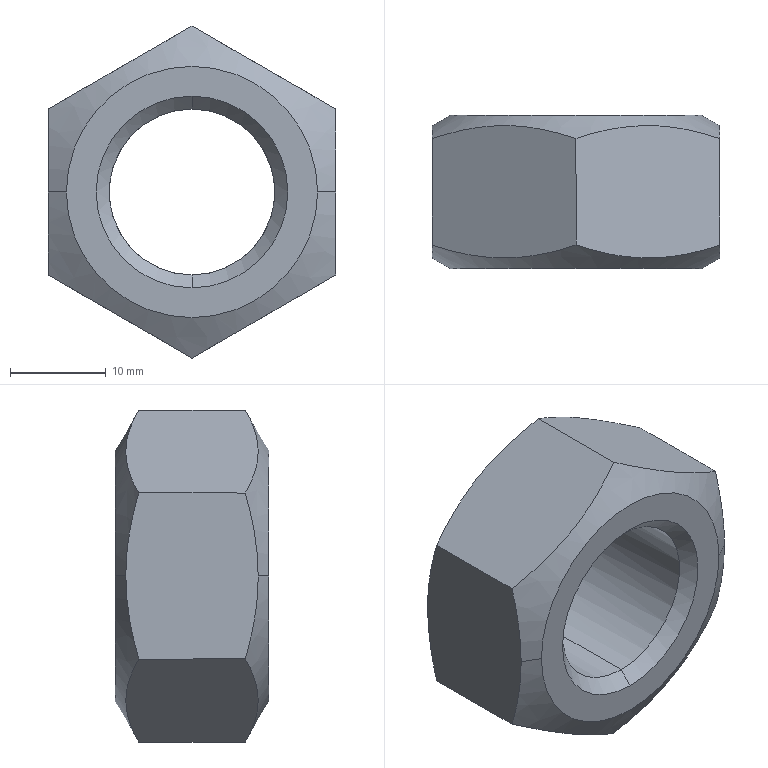Part | SolidWorks | features BaseBody 1 | 1 solid | 18 faces | box 30 x 16 x 34.641 mm | volume 8202 mm3 | cone 8 | plane 8 | cylinder 2 | commonest cylinder face diameters 17.294 x2
STEP:
#1=CARTESIAN_POINT('',(0.,94.353,-8.647));
#2=VERTEX_POINT('',#1);
#3=CARTESIAN_POINT('',(0.,94.353,8.647));
#4=VERTEX_POINT('',#3);
#5=CARTESIAN_POINT('',(0.,94.353,0.));
#6=DIRECTION('',(0.,1.,0.));
#7=DIRECTION('',(0.,0.,1.));
#8=AXIS2_PLACEMENT_3D('',#5,#6,#7);
#9=CIRCLE('',#8,8.647);
#10=EDGE_CURVE('',#2,#4,#9,.T.);
#11=ORIENTED_EDGE('',*,*,#10,.F.);
#12=CARTESIAN_POINT('',(0.,107.647,-8.647));
#13=VERTEX_POINT('',#12);
#14=CARTESIAN_POINT('',(0.,500.,-8.647));
#15=DIRECTION('',(0.,1.,0.));
#16=VECTOR('',#15,1000.);
#17=LINE('',#14,#16);
#18=EDGE_CURVE('',#2,#13,#17,.T.);
#19=ORIENTED_EDGE('',*,*,#18,.T.);
#20=CARTESIAN_POINT('',(-8.647,107.647,0.));
#21=VERTEX_POINT('',#20);
#22=CARTESIAN_POINT('',(0.,107.647,0.));
#23=DIRECTION('',(0.,-1.,0.));
#24=DIRECTION('',(0.,0.,1.));
#25=AXIS2_PLACEMENT_3D('',#22,#23,#24);
#26=CIRCLE('',#25,8.647);
#27=EDGE_CURVE('',#21,#13,#26,.T.);
#28=ORIENTED_EDGE('',*,*,#27,.F.);
#29=CARTESIAN_POINT('',(0.,107.647,8.647));
#30=VERTEX_POINT('',#29);
#31=CARTESIAN_POINT('',(0.,107.647,0.));
#32=DIRECTION('',(0.,-1.,0.));
#33=DIRECTION('',(0.,0.,1.));
#34=AXIS2_PLACEMENT_3D('',#31,#32,#33);
#35=CIRCLE('',#34,8.647);
#36=EDGE_CURVE('',#30,#21,#35,.T.);
#37=ORIENTED_EDGE('',*,*,#36,.F.);
#38=CARTESIAN_POINT('',(0.,500.,8.647));
#39=DIRECTION('',(0.,1.,0.));
#40=VECTOR('',#39,1000.);
#41=LINE('',#38,#40);
#42=EDGE_CURVE('',#4,#30,#41,.T.);
#43=ORIENTED_EDGE('',*,*,#42,.F.);
#44=EDGE_LOOP('',(#11,#19,#28,#37,#43));
#45=FACE_OUTER_BOUND('',#44,.T.);
#46=CARTESIAN_POINT('',(0.,500.,0.));
#47=DIRECTION('',(0.,1.,0.));
#48=DIRECTION('',(0.,0.,1.));
#49=AXIS2_PLACEMENT_3D('',#46,#47,#48);
#50=CYLINDRICAL_SURFACE('',#49,8.647);
#51=ADVANCED_FACE('',(#45),#50,.F.);
#52=ORIENTED_EDGE('',*,*,#10,.T.);
#53=CARTESIAN_POINT('',(0.,93.,10.));
#54=VERTEX_POINT('',#53);
#55=CARTESIAN_POINT('',(0.,93.,10.));
#56=DIRECTION('',(0.,-0.7071,0.7071));
#57=VECTOR('',#56,1000.);
#58=LINE('',#55,#57);
#59=EDGE_CURVE('',#4,#54,#58,.T.);
#60=ORIENTED_EDGE('',*,*,#59,.T.);
#61=CARTESIAN_POINT('',(0.,93.,-10.));
#62=VERTEX_POINT('',#61);
#63=CARTESIAN_POINT('',(0.,93.,0.));
#64=DIRECTION('',(0.,1.,0.));
#65=DIRECTION('',(0.,0.,-1.));
#66=AXIS2_PLACEMENT_3D('',#63,#64,#65);
#67=CIRCLE('',#66,10.);
#68=EDGE_CURVE('',#62,#54,#67,.T.);
#69=ORIENTED_EDGE('',*,*,#68,.F.);
#70=CARTESIAN_POINT('',(0.,93.,-10.));
#71=DIRECTION('',(0.,-0.7071,-0.7071));
#72=VECTOR('',#71,1000.);
#73=LINE('',#70,#72);
#74=EDGE_CURVE('',#2,#62,#73,.T.);
#75=ORIENTED_EDGE('',*,*,#74,.F.);
#76=EDGE_LOOP('',(#52,#60,#69,#75));
#77=FACE_OUTER_BOUND('',#76,.T.);
#78=CARTESIAN_POINT('',(0.,93.,0.));
#79=DIRECTION('',(0.,-1.,0.));
#80=DIRECTION('',(0.,0.,-1.));
#81=AXIS2_PLACEMENT_3D('',#78,#79,#80);
#82=CONICAL_SURFACE('',#81,10.,0.7854);
#83=ADVANCED_FACE('',(#77),#82,.F.);
#84=ORIENTED_EDGE('',*,*,#27,.T.);
#85=CARTESIAN_POINT('',(8.647,107.647,0.));
#86=VERTEX_POINT('',#85);
#87=CARTESIAN_POINT('',(0.,107.647,0.));
#88=DIRECTION('',(0.,-1.,0.));
#89=DIRECTION('',(0.,0.,1.));
#90=AXIS2_PLACEMENT_3D('',#87,#88,#89);
#91=CIRCLE('',#90,8.647);
#92=EDGE_CURVE('',#13,#86,#91,.T.);
#93=ORIENTED_EDGE('',*,*,#92,.T.);
#94=CARTESIAN_POINT('',(10.,109.,0.));
#95=VERTEX_POINT('',#94);
#96=CARTESIAN_POINT('',(10.,109.,0.));
#97=DIRECTION('',(0.7071,0.7071,0.));
#98=VECTOR('',#97,1000.);
#99=LINE('',#96,#98);
#100=EDGE_CURVE('',#86,#95,#99,.T.);
#101=ORIENTED_EDGE('',*,*,#100,.T.);
#102=CARTESIAN_POINT('',(-10.,109.,0.));
#103=VERTEX_POINT('',#102);
#104=CARTESIAN_POINT('',(0.,109.,0.));
#105=DIRECTION('',(0.,-1.,0.));
#106=DIRECTION('',(-1.,0.,0.));
#107=AXIS2_PLACEMENT_3D('',#104,#105,#106);
#108=CIRCLE('',#107,10.);
#109=EDGE_CURVE('',#103,#95,#108,.T.);
#110=ORIENTED_EDGE('',*,*,#109,.F.);
#111=CARTESIAN_POINT('',(-10.,109.,0.));
#112=DIRECTION('',(-0.7071,0.7071,0.));
#113=VECTOR('',#112,1000.);
#114=LINE('',#111,#113);
#115=EDGE_CURVE('',#21,#103,#114,.T.);
#116=ORIENTED_EDGE('',*,*,#115,.F.);
#117=EDGE_LOOP('',(#84,#93,#101,#110,#116));
#118=FACE_OUTER_BOUND('',#117,.T.);
#119=CARTESIAN_POINT('',(0.,109.,0.));
#120=DIRECTION('',(0.,1.,0.));
#121=DIRECTION('',(-1.,0.,0.));
#122=AXIS2_PLACEMENT_3D('',#119,#120,#121);
#123=CONICAL_SURFACE('',#122,10.,0.7854);
#124=ADVANCED_FACE('',(#118),#123,.F.);
#125=CARTESIAN_POINT('',(13.1,93.,0.));
#126=VERTEX_POINT('',#125);
#127=CARTESIAN_POINT('',(-13.1,93.,0.));
#128=VERTEX_POINT('',#127);
#129=CARTESIAN_POINT('',(0.,93.,0.));
#130=DIRECTION('',(0.,-1.,0.));
#131=DIRECTION('',(-1.,0.,0.));
#132=AXIS2_PLACEMENT_3D('',#129,#130,#131);
#133=CIRCLE('',#132,13.1);
#134=EDGE_CURVE('',#126,#128,#133,.T.);
#135=ORIENTED_EDGE('',*,*,#134,.F.);
#136=CARTESIAN_POINT('',(15.,94.097,0.));
#137=VERTEX_POINT('',#136);
#138=CARTESIAN_POINT('',(17.346,95.451,0.));
#139=DIRECTION('',(0.866,0.5,0.));
#140=VECTOR('',#139,1000.);
#141=LINE('',#138,#140);
#142=EDGE_CURVE('',#126,#137,#141,.T.);
#143=ORIENTED_EDGE('',*,*,#142,.T.);
#144=CARTESIAN_POINT('',(15.,95.437,8.66));
#145=VERTEX_POINT('',#144);
#146=CARTESIAN_POINT('',(15.,94.097,0.));
#147=CARTESIAN_POINT('',(15.,94.097,0.735));
#148=CARTESIAN_POINT('',(15.,94.129,1.473));
#149=CARTESIAN_POINT('',(15.,94.251,2.934));
#150=CARTESIAN_POINT('',(15.,94.342,3.659));
#151=CARTESIAN_POINT('',(15.,94.692,5.822));
#152=CARTESIAN_POINT('',(15.,95.029,7.247));
#153=CARTESIAN_POINT('',(15.,95.437,8.66));
#154=B_SPLINE_CURVE_WITH_KNOTS('',3,(#146,#147,#148,#149,#150,#151,#152,#153),.UNSPECIFIED.,.F.,.F.,(4,2,2,4),(0.008763,0.01095,0.01313,0.01749),.UNSPECIFIED.);
#155=EDGE_CURVE('',#137,#145,#154,.T.);
#156=ORIENTED_EDGE('',*,*,#155,.T.);
#157=CARTESIAN_POINT('',(0.000000043,95.437,17.321));
#158=VERTEX_POINT('',#157);
#159=CARTESIAN_POINT('',(15.,95.437,8.66));
#160=CARTESIAN_POINT('',(13.775,95.029,9.367));
#161=CARTESIAN_POINT('',(12.542,94.692,10.079));
#162=CARTESIAN_POINT('',(10.049,94.226,11.519));
#163=CARTESIAN_POINT('',(8.79,94.098,12.246));
#164=CARTESIAN_POINT('',(6.877,94.097,13.35));
#165=CARTESIAN_POINT('',(6.236,94.128,13.72));
#166=CARTESIAN_POINT('',(4.969,94.25,14.452));
#167=CARTESIAN_POINT('',(4.339,94.341,14.815));
#168=CARTESIAN_POINT('',(2.463,94.691,15.899));
#169=CARTESIAN_POINT('',(1.226,95.028,16.613));
#170=CARTESIAN_POINT('',(0.000000043,95.437,17.321));
#171=B_SPLINE_CURVE_WITH_KNOTS('',3,(#159,#160,#161,#162,#163,#164,#165,#166,#167,#168,#169,#170),.UNSPECIFIED.,.F.,.F.,(4,2,2,2,2,4),(0.,0.004373,0.008746,0.01093,0.01312,0.01749),.UNSPECIFIED.);
#172=EDGE_CURVE('',#145,#158,#171,.T.);
#173=ORIENTED_EDGE('',*,*,#172,.T.);
#174=CARTESIAN_POINT('',(-15.,95.437,8.66));
#175=VERTEX_POINT('',#174);
#176=CARTESIAN_POINT('',(0.000000043,95.437,17.321));
#177=CARTESIAN_POINT('',(-1.225,95.029,16.613));
#178=CARTESIAN_POINT('',(-2.458,94.692,15.901));
#179=CARTESIAN_POINT('',(-4.951,94.226,14.462));
#180=CARTESIAN_POINT('',(-6.21,94.098,13.735));
#181=CARTESIAN_POINT('',(-8.123,94.097,12.631));
#182=CARTESIAN_POINT('',(-8.764,94.128,12.261));
#183=CARTESIAN_POINT('',(-10.031,94.25,11.529));
#184=CARTESIAN_POINT('',(-10.661,94.341,11.166));
#185=CARTESIAN_POINT('',(-12.537,94.691,10.082));
#186=CARTESIAN_POINT('',(-13.774,95.028,9.368));
#187=CARTESIAN_POINT('',(-15.,95.437,8.66));
#188=B_SPLINE_CURVE_WITH_KNOTS('',3,(#176,#177,#178,#179,#180,#181,#182,#183,#184,#185,#186,#187),.UNSPECIFIED.,.F.,.F.,(4,2,2,2,2,4),(0.,0.004373,0.008746,0.01093,0.01312,0.01749),.UNSPECIFIED.);
#189=EDGE_CURVE('',#158,#175,#188,.T.);
#190=ORIENTED_EDGE('',*,*,#189,.T.);
#191=CARTESIAN_POINT('',(-15.,94.097,0.));
#192=VERTEX_POINT('',#191);
#193=CARTESIAN_POINT('',(-15.,95.437,8.66));
#194=CARTESIAN_POINT('',(-15.,95.028,7.244));
#195=CARTESIAN_POINT('',(-15.,94.691,5.816));
#196=CARTESIAN_POINT('',(-15.,94.225,2.933));
#197=CARTESIAN_POINT('',(-15.,94.097,1.475));
#198=CARTESIAN_POINT('',(-15.,94.097,0.));
#199=B_SPLINE_CURVE_WITH_KNOTS('',3,(#193,#194,#195,#196,#197,#198),.UNSPECIFIED.,.F.,.F.,(4,2,4),(0.,0.004381,0.008763),.UNSPECIFIED.);
#200=EDGE_CURVE('',#175,#192,#199,.T.);
#201=ORIENTED_EDGE('',*,*,#200,.T.);
#202=CARTESIAN_POINT('',(-17.346,95.451,0.));
#203=DIRECTION('',(-0.866,0.5,0.));
#204=VECTOR('',#203,1000.);
#205=LINE('',#202,#204);
#206=EDGE_CURVE('',#128,#192,#205,.T.);
#207=ORIENTED_EDGE('',*,*,#206,.F.);
#208=EDGE_LOOP('',(#135,#143,#156,#173,#190,#201,#207));
#209=FACE_OUTER_BOUND('',#208,.T.);
#210=CARTESIAN_POINT('',(0.,95.451,0.));
#211=DIRECTION('',(0.,1.,0.));
#212=DIRECTION('',(-1.,0.,0.));
#213=AXIS2_PLACEMENT_3D('',#210,#211,#212);
#214=CONICAL_SURFACE('',#213,17.346,1.047);
#215=ADVANCED_FACE('',(#209),#214,.T.);
#216=CARTESIAN_POINT('',(-13.1,109.,0.));
#217=VERTEX_POINT('',#216);
#218=CARTESIAN_POINT('',(13.1,109.,0.));
#219=VERTEX_POINT('',#218);
#220=CARTESIAN_POINT('',(0.,109.,0.));
#221=DIRECTION('',(0.,1.,0.));
#222=DIRECTION('',(1.,0.,0.));
#223=AXIS2_PLACEMENT_3D('',#220,#221,#222);
#224=CIRCLE('',#223,13.1);
#225=EDGE_CURVE('',#217,#219,#224,.T.);
#226=ORIENTED_EDGE('',*,*,#225,.F.);
#227=CARTESIAN_POINT('',(-15.,107.903,0.));
#228=VERTEX_POINT('',#227);
#229=CARTESIAN_POINT('',(-17.346,106.549,0.));
#230=DIRECTION('',(-0.866,-0.5,0.));
#231=VECTOR('',#230,1000.);
#232=LINE('',#229,#231);
#233=EDGE_CURVE('',#217,#228,#232,.T.);
#234=ORIENTED_EDGE('',*,*,#233,.T.);
#235=CARTESIAN_POINT('',(-15.,106.563,8.66));
#236=VERTEX_POINT('',#235);
#237=CARTESIAN_POINT('',(-15.,107.903,0.));
#238=CARTESIAN_POINT('',(-15.,107.903,0.735));
#239=CARTESIAN_POINT('',(-15.,107.871,1.473));
#240=CARTESIAN_POINT('',(-15.,107.749,2.934));
#241=CARTESIAN_POINT('',(-15.,107.658,3.659));
#242=CARTESIAN_POINT('',(-15.,107.308,5.822));
#243=CARTESIAN_POINT('',(-15.,106.971,7.247));
#244=CARTESIAN_POINT('',(-15.,106.563,8.66));
#245=B_SPLINE_CURVE_WITH_KNOTS('',3,(#237,#238,#239,#240,#241,#242,#243,#244),.UNSPECIFIED.,.F.,.F.,(4,2,2,4),(0.008763,0.01095,0.01313,0.01749),.UNSPECIFIED.);
#246=EDGE_CURVE('',#228,#236,#245,.T.);
#247=ORIENTED_EDGE('',*,*,#246,.T.);
#248=CARTESIAN_POINT('',(-0.000000043,106.563,17.321));
#249=VERTEX_POINT('',#248);
#250=CARTESIAN_POINT('',(-15.,106.563,8.66));
#251=CARTESIAN_POINT('',(-13.775,106.971,9.367));
#252=CARTESIAN_POINT('',(-12.542,107.308,10.079));
#253=CARTESIAN_POINT('',(-10.049,107.774,11.519));
#254=CARTESIAN_POINT('',(-8.79,107.902,12.246));
#255=CARTESIAN_POINT('',(-6.877,107.903,13.35));
#256=CARTESIAN_POINT('',(-6.236,107.872,13.72));
#257=CARTESIAN_POINT('',(-4.969,107.75,14.452));
#258=CARTESIAN_POINT('',(-4.339,107.659,14.815));
#259=CARTESIAN_POINT('',(-2.463,107.309,15.899));
#260=CARTESIAN_POINT('',(-1.226,106.972,16.613));
#261=CARTESIAN_POINT('',(-0.000000043,106.563,17.321));
#262=B_SPLINE_CURVE_WITH_KNOTS('',3,(#250,#251,#252,#253,#254,#255,#256,#257,#258,#259,#260,#261),.UNSPECIFIED.,.F.,.F.,(4,2,2,2,2,4),(0.,0.004373,0.008746,0.01093,0.01312,0.01749),.UNSPECIFIED.);
#263=EDGE_CURVE('',#236,#249,#262,.T.);
#264=ORIENTED_EDGE('',*,*,#263,.T.);
#265=CARTESIAN_POINT('',(15.,106.563,8.66));
#266=VERTEX_POINT('',#265);
#267=CARTESIAN_POINT('',(-0.000000043,106.563,17.321));
#268=CARTESIAN_POINT('',(1.225,106.971,16.613));
#269=CARTESIAN_POINT('',(2.458,107.308,15.901));
#270=CARTESIAN_POINT('',(4.951,107.774,14.462));
#271=CARTESIAN_POINT('',(6.21,107.902,13.735));
#272=CARTESIAN_POINT('',(8.123,107.903,12.631));
#273=CARTESIAN_POINT('',(8.764,107.872,12.261));
#274=CARTESIAN_POINT('',(10.031,107.75,11.529));
#275=CARTESIAN_POINT('',(10.661,107.659,11.166));
#276=CARTESIAN_POINT('',(12.537,107.309,10.082));
#277=CARTESIAN_POINT('',(13.774,106.972,9.368));
#278=CARTESIAN_POINT('',(15.,106.563,8.66));
#279=B_SPLINE_CURVE_WITH_KNOTS('',3,(#267,#268,#269,#270,#271,#272,#273,#274,#275,#276,#277,#278),.UNSPECIFIED.,.F.,.F.,(4,2,2,2,2,4),(0.,0.004373,0.008746,0.01093,0.01312,0.01749),.UNSPECIFIED.);
#280=EDGE_CURVE('',#249,#266,#279,.T.);
#281=ORIENTED_EDGE('',*,*,#280,.T.);
#282=CARTESIAN_POINT('',(15.,107.903,0.));
#283=VERTEX_POINT('',#282);
#284=CARTESIAN_POINT('',(15.,106.563,8.66));
#285=CARTESIAN_POINT('',(15.,106.972,7.244));
#286=CARTESIAN_POINT('',(15.,107.309,5.816));
#287=CARTESIAN_POINT('',(15.,107.775,2.933));
#288=CARTESIAN_POINT('',(15.,107.903,1.475));
#289=CARTESIAN_POINT('',(15.,107.903,0.));
#290=B_SPLINE_CURVE_WITH_KNOTS('',3,(#284,#285,#286,#287,#288,#289),.UNSPECIFIED.,.F.,.F.,(4,2,4),(0.,0.004381,0.008763),.UNSPECIFIED.);
#291=EDGE_CURVE('',#266,#283,#290,.T.);
#292=ORIENTED_EDGE('',*,*,#291,.T.);
#293=CARTESIAN_POINT('',(17.346,106.549,0.));
#294=DIRECTION('',(0.866,-0.5,0.));
#295=VECTOR('',#294,1000.);
#296=LINE('',#293,#295);
#297=EDGE_CURVE('',#219,#283,#296,.T.);
#298=ORIENTED_EDGE('',*,*,#297,.F.);
#299=EDGE_LOOP('',(#226,#234,#247,#264,#281,#292,#298));
#300=FACE_OUTER_BOUND('',#299,.T.);
#301=CARTESIAN_POINT('',(0.,106.549,0.));
#302=DIRECTION('',(0.,-1.,0.));
#303=DIRECTION('',(1.,0.,0.));
#304=AXIS2_PLACEMENT_3D('',#301,#302,#303);
#305=CONICAL_SURFACE('',#304,17.346,1.047);
#306=ADVANCED_FACE('',(#300),#305,.T.);
#307=ORIENTED_EDGE('',*,*,#18,.F.);
#308=CARTESIAN_POINT('',(0.,94.353,0.));
#309=DIRECTION('',(0.,1.,0.));
#310=DIRECTION('',(0.,0.,1.));
#311=AXIS2_PLACEMENT_3D('',#308,#309,#310);
#312=CIRCLE('',#311,8.647);
#313=EDGE_CURVE('',#4,#2,#312,.T.);
#314=ORIENTED_EDGE('',*,*,#313,.F.);
#315=ORIENTED_EDGE('',*,*,#42,.T.);
#316=CARTESIAN_POINT('',(0.,107.647,0.));
#317=DIRECTION('',(0.,-1.,0.));
#318=DIRECTION('',(0.,0.,1.));
#319=AXIS2_PLACEMENT_3D('',#316,#317,#318);
#320=CIRCLE('',#319,8.647);
#321=EDGE_CURVE('',#86,#30,#320,.T.);
#322=ORIENTED_EDGE('',*,*,#321,.F.);
#323=ORIENTED_EDGE('',*,*,#92,.F.);
#324=EDGE_LOOP('',(#307,#314,#315,#322,#323));
#325=FACE_OUTER_BOUND('',#324,.T.);
#326=CARTESIAN_POINT('',(0.,500.,0.));
#327=DIRECTION('',(0.,1.,0.));
#328=DIRECTION('',(0.,0.,1.));
#329=AXIS2_PLACEMENT_3D('',#326,#327,#328);
#330=CYLINDRICAL_SURFACE('',#329,8.647);
#331=ADVANCED_FACE('',(#325),#330,.F.);
#332=ORIENTED_EDGE('',*,*,#59,.F.);
#333=ORIENTED_EDGE('',*,*,#313,.T.);
#334=ORIENTED_EDGE('',*,*,#74,.T.);
#335=CARTESIAN_POINT('',(0.,93.,0.));
#336=DIRECTION('',(0.,1.,0.));
#337=DIRECTION('',(0.,0.,-1.));
#338=AXIS2_PLACEMENT_3D('',#335,#336,#337);
#339=CIRCLE('',#338,10.);
#340=EDGE_CURVE('',#54,#62,#339,.T.);
#341=ORIENTED_EDGE('',*,*,#340,.F.);
#342=EDGE_LOOP('',(#332,#333,#334,#341));
#343=FACE_OUTER_BOUND('',#342,.T.);
#344=CARTESIAN_POINT('',(0.,93.,0.));
#345=DIRECTION('',(0.,-1.,0.));
#346=DIRECTION('',(0.,0.,-1.));
#347=AXIS2_PLACEMENT_3D('',#344,#345,#346);
#348=CONICAL_SURFACE('',#347,10.,0.7854);
#349=ADVANCED_FACE('',(#343),#348,.F.);
#350=ORIENTED_EDGE('',*,*,#100,.F.);
#351=ORIENTED_EDGE('',*,*,#321,.T.);
#352=ORIENTED_EDGE('',*,*,#36,.T.);
#353=ORIENTED_EDGE('',*,*,#115,.T.);
#354=CARTESIAN_POINT('',(0.,109.,0.));
#355=DIRECTION('',(0.,-1.,0.));
#356=DIRECTION('',(-1.,0.,0.));
#357=AXIS2_PLACEMENT_3D('',#354,#355,#356);
#358=CIRCLE('',#357,10.);
#359=EDGE_CURVE('',#95,#103,#358,.T.);
#360=ORIENTED_EDGE('',*,*,#359,.F.);
#361=EDGE_LOOP('',(#350,#351,#352,#353,#360));
#362=FACE_OUTER_BOUND('',#361,.T.);
#363=CARTESIAN_POINT('',(0.,109.,0.));
#364=DIRECTION('',(0.,1.,0.));
#365=DIRECTION('',(-1.,0.,0.));
#366=AXIS2_PLACEMENT_3D('',#363,#364,#365);
#367=CONICAL_SURFACE('',#366,10.,0.7854);
#368=ADVANCED_FACE('',(#362),#367,.F.);
#369=CARTESIAN_POINT('',(0.,93.,0.));
#370=DIRECTION('',(0.,-1.,0.));
#371=DIRECTION('',(-1.,0.,0.));
#372=AXIS2_PLACEMENT_3D('',#369,#370,#371);
#373=CIRCLE('',#372,13.1);
#374=EDGE_CURVE('',#128,#126,#373,.T.);
#375=ORIENTED_EDGE('',*,*,#374,.T.);
#376=ORIENTED_EDGE('',*,*,#134,.T.);
#377=EDGE_LOOP('',(#375,#376));
#378=FACE_OUTER_BOUND('',#377,.T.);
#379=ORIENTED_EDGE('',*,*,#68,.T.);
#380=ORIENTED_EDGE('',*,*,#340,.T.);
#381=EDGE_LOOP('',(#379,#380));
#382=FACE_BOUND('',#381,.T.);
#383=CARTESIAN_POINT('',(0.,93.,13.1));
#384=DIRECTION('',(0.,-1.,0.));
#385=DIRECTION('',(0.,0.,-1.));
#386=AXIS2_PLACEMENT_3D('',#383,#384,#385);
#387=PLANE('',#386);
#388=ADVANCED_FACE('',(#378,#382),#387,.T.);
#389=ORIENTED_EDGE('',*,*,#109,.T.);
#390=ORIENTED_EDGE('',*,*,#359,.T.);
#391=EDGE_LOOP('',(#389,#390));
#392=FACE_BOUND('',#391,.T.);
#393=CARTESIAN_POINT('',(0.,109.,0.));
#394=DIRECTION('',(0.,1.,0.));
#395=DIRECTION('',(1.,0.,0.));
#396=AXIS2_PLACEMENT_3D('',#393,#394,#395);
#397=CIRCLE('',#396,13.1);
#398=EDGE_CURVE('',#219,#217,#397,.T.);
#399=ORIENTED_EDGE('',*,*,#398,.T.);
#400=ORIENTED_EDGE('',*,*,#225,.T.);
#401=EDGE_LOOP('',(#399,#400));
#402=FACE_OUTER_BOUND('',#401,.T.);
#403=CARTESIAN_POINT('',(0.,109.,10.));
#404=DIRECTION('',(0.,1.,0.));
#405=DIRECTION('',(0.,0.,1.));
#406=AXIS2_PLACEMENT_3D('',#403,#404,#405);
#407=PLANE('',#406);
#408=ADVANCED_FACE('',(#392,#402),#407,.T.);
#409=ORIENTED_EDGE('',*,*,#142,.F.);
#410=ORIENTED_EDGE('',*,*,#374,.F.);
#411=ORIENTED_EDGE('',*,*,#206,.T.);
#412=CARTESIAN_POINT('',(-15.,95.437,-8.66));
#413=VERTEX_POINT('',#412);
#414=CARTESIAN_POINT('',(-15.,94.097,0.));
#415=CARTESIAN_POINT('',(-15.,94.097,-0.735));
#416=CARTESIAN_POINT('',(-15.,94.129,-1.473));
#417=CARTESIAN_POINT('',(-15.,94.251,-2.934));
#418=CARTESIAN_POINT('',(-15.,94.342,-3.659));
#419=CARTESIAN_POINT('',(-15.,94.692,-5.822));
#420=CARTESIAN_POINT('',(-15.,95.029,-7.247));
#421=CARTESIAN_POINT('',(-15.,95.437,-8.66));
#422=B_SPLINE_CURVE_WITH_KNOTS('',3,(#414,#415,#416,#417,#418,#419,#420,#421),.UNSPECIFIED.,.F.,.F.,(4,2,2,4),(0.008763,0.01095,0.01313,0.01749),.UNSPECIFIED.);
#423=EDGE_CURVE('',#192,#413,#422,.T.);
#424=ORIENTED_EDGE('',*,*,#423,.T.);
#425=CARTESIAN_POINT('',(-0.000000043,95.437,-17.321));
#426=VERTEX_POINT('',#425);
#427=CARTESIAN_POINT('',(-15.,95.437,-8.66));
#428=CARTESIAN_POINT('',(-13.775,95.029,-9.367));
#429=CARTESIAN_POINT('',(-12.542,94.692,-10.079));
#430=CARTESIAN_POINT('',(-10.049,94.226,-11.519));
#431=CARTESIAN_POINT('',(-8.79,94.098,-12.246));
#432=CARTESIAN_POINT('',(-6.877,94.097,-13.35));
#433=CARTESIAN_POINT('',(-6.236,94.128,-13.72));
#434=CARTESIAN_POINT('',(-4.969,94.25,-14.452));
#435=CARTESIAN_POINT('',(-4.339,94.341,-14.815));
#436=CARTESIAN_POINT('',(-2.463,94.691,-15.899));
#437=CARTESIAN_POINT('',(-1.226,95.028,-16.613));
#438=CARTESIAN_POINT('',(-0.000000043,95.437,-17.321));
#439=B_SPLINE_CURVE_WITH_KNOTS('',3,(#427,#428,#429,#430,#431,#432,#433,#434,#435,#436,#437,#438),.UNSPECIFIED.,.F.,.F.,(4,2,2,2,2,4),(0.,0.004373,0.008746,0.01093,0.01312,0.01749),.UNSPECIFIED.);
#440=EDGE_CURVE('',#413,#426,#439,.T.);
#441=ORIENTED_EDGE('',*,*,#440,.T.);
#442=CARTESIAN_POINT('',(15.,95.437,-8.66));
#443=VERTEX_POINT('',#442);
#444=CARTESIAN_POINT('',(-0.000000043,95.437,-17.321));
#445=CARTESIAN_POINT('',(1.225,95.029,-16.613));
#446=CARTESIAN_POINT('',(2.458,94.692,-15.901));
#447=CARTESIAN_POINT('',(4.951,94.226,-14.462));
#448=CARTESIAN_POINT('',(6.21,94.098,-13.735));
#449=CARTESIAN_POINT('',(8.123,94.097,-12.631));
#450=CARTESIAN_POINT('',(8.764,94.128,-12.261));
#451=CARTESIAN_POINT('',(10.031,94.25,-11.529));
#452=CARTESIAN_POINT('',(10.661,94.341,-11.166));
#453=CARTESIAN_POINT('',(12.537,94.691,-10.082));
#454=CARTESIAN_POINT('',(13.774,95.028,-9.368));
#455=CARTESIAN_POINT('',(15.,95.437,-8.66));
#456=B_SPLINE_CURVE_WITH_KNOTS('',3,(#444,#445,#446,#447,#448,#449,#450,#451,#452,#453,#454,#455),.UNSPECIFIED.,.F.,.F.,(4,2,2,2,2,4),(0.,0.004373,0.008746,0.01093,0.01312,0.01749),.UNSPECIFIED.);
#457=EDGE_CURVE('',#426,#443,#456,.T.);
#458=ORIENTED_EDGE('',*,*,#457,.T.);
#459=CARTESIAN_POINT('',(15.,95.437,-8.66));
#460=CARTESIAN_POINT('',(15.,95.028,-7.244));
#461=CARTESIAN_POINT('',(15.,94.691,-5.816));
#462=CARTESIAN_POINT('',(15.,94.225,-2.933));
#463=CARTESIAN_POINT('',(15.,94.097,-1.475));
#464=CARTESIAN_POINT('',(15.,94.097,0.));
#465=B_SPLINE_CURVE_WITH_KNOTS('',3,(#459,#460,#461,#462,#463,#464),.UNSPECIFIED.,.F.,.F.,(4,2,4),(0.,0.004381,0.008763),.UNSPECIFIED.);
#466=EDGE_CURVE('',#443,#137,#465,.T.);
#467=ORIENTED_EDGE('',*,*,#466,.T.);
#468=EDGE_LOOP('',(#409,#410,#411,#424,#441,#458,#467));
#469=FACE_OUTER_BOUND('',#468,.T.);
#470=CARTESIAN_POINT('',(0.,95.451,0.));
#471=DIRECTION('',(0.,1.,0.));
#472=DIRECTION('',(-1.,0.,0.));
#473=AXIS2_PLACEMENT_3D('',#470,#471,#472);
#474=CONICAL_SURFACE('',#473,17.346,1.047);
#475=ADVANCED_FACE('',(#469),#474,.T.);
#476=ORIENTED_EDGE('',*,*,#233,.F.);
#477=ORIENTED_EDGE('',*,*,#398,.F.);
#478=ORIENTED_EDGE('',*,*,#297,.T.);
#479=CARTESIAN_POINT('',(15.,106.563,-8.66));
#480=VERTEX_POINT('',#479);
#481=CARTESIAN_POINT('',(15.,107.903,0.));
#482=CARTESIAN_POINT('',(15.,107.903,-0.735));
#483=CARTESIAN_POINT('',(15.,107.871,-1.473));
#484=CARTESIAN_POINT('',(15.,107.749,-2.934));
#485=CARTESIAN_POINT('',(15.,107.658,-3.659));
#486=CARTESIAN_POINT('',(15.,107.308,-5.822));
#487=CARTESIAN_POINT('',(15.,106.971,-7.247));
#488=CARTESIAN_POINT('',(15.,106.563,-8.66));
#489=B_SPLINE_CURVE_WITH_KNOTS('',3,(#481,#482,#483,#484,#485,#486,#487,#488),.UNSPECIFIED.,.F.,.F.,(4,2,2,4),(0.008763,0.01095,0.01313,0.01749),.UNSPECIFIED.);
#490=EDGE_CURVE('',#283,#480,#489,.T.);
#491=ORIENTED_EDGE('',*,*,#490,.T.);
#492=CARTESIAN_POINT('',(0.000000043,106.563,-17.321));
#493=VERTEX_POINT('',#492);
#494=CARTESIAN_POINT('',(15.,106.563,-8.66));
#495=CARTESIAN_POINT('',(13.775,106.971,-9.367));
#496=CARTESIAN_POINT('',(12.542,107.308,-10.079));
#497=CARTESIAN_POINT('',(10.049,107.774,-11.519));
#498=CARTESIAN_POINT('',(8.79,107.902,-12.246));
#499=CARTESIAN_POINT('',(6.877,107.903,-13.35));
#500=CARTESIAN_POINT('',(6.236,107.872,-13.72));
#501=CARTESIAN_POINT('',(4.969,107.75,-14.452));
#502=CARTESIAN_POINT('',(4.339,107.659,-14.815));
#503=CARTESIAN_POINT('',(2.463,107.309,-15.899));
#504=CARTESIAN_POINT('',(1.226,106.972,-16.613));
#505=CARTESIAN_POINT('',(0.000000043,106.563,-17.321));
#506=B_SPLINE_CURVE_WITH_KNOTS('',3,(#494,#495,#496,#497,#498,#499,#500,#501,#502,#503,#504,#505),.UNSPECIFIED.,.F.,.F.,(4,2,2,2,2,4),(0.,0.004373,0.008746,0.01093,0.01312,0.01749),.UNSPECIFIED.);
#507=EDGE_CURVE('',#480,#493,#506,.T.);
#508=ORIENTED_EDGE('',*,*,#507,.T.);
#509=CARTESIAN_POINT('',(-15.,106.563,-8.66));
#510=VERTEX_POINT('',#509);
#511=CARTESIAN_POINT('',(0.000000043,106.563,-17.321));
#512=CARTESIAN_POINT('',(-1.225,106.971,-16.613));
#513=CARTESIAN_POINT('',(-2.458,107.308,-15.901));
#514=CARTESIAN_POINT('',(-4.951,107.774,-14.462));
#515=CARTESIAN_POINT('',(-6.21,107.902,-13.735));
#516=CARTESIAN_POINT('',(-8.123,107.903,-12.631));
#517=CARTESIAN_POINT('',(-8.764,107.872,-12.261));
#518=CARTESIAN_POINT('',(-10.031,107.75,-11.529));
#519=CARTESIAN_POINT('',(-10.661,107.659,-11.166));
#520=CARTESIAN_POINT('',(-12.537,107.309,-10.082));
#521=CARTESIAN_POINT('',(-13.774,106.972,-9.368));
#522=CARTESIAN_POINT('',(-15.,106.563,-8.66));
#523=B_SPLINE_CURVE_WITH_KNOTS('',3,(#511,#512,#513,#514,#515,#516,#517,#518,#519,#520,#521,#522),.UNSPECIFIED.,.F.,.F.,(4,2,2,2,2,4),(0.,0.004373,0.008746,0.01093,0.01312,0.01749),.UNSPECIFIED.);
#524=EDGE_CURVE('',#493,#510,#523,.T.);
#525=ORIENTED_EDGE('',*,*,#524,.T.);
#526=CARTESIAN_POINT('',(-15.,106.563,-8.66));
#527=CARTESIAN_POINT('',(-15.,106.972,-7.244));
#528=CARTESIAN_POINT('',(-15.,107.309,-5.816));
#529=CARTESIAN_POINT('',(-15.,107.775,-2.933));
#530=CARTESIAN_POINT('',(-15.,107.903,-1.475));
#531=CARTESIAN_POINT('',(-15.,107.903,0.));
#532=B_SPLINE_CURVE_WITH_KNOTS('',3,(#526,#527,#528,#529,#530,#531),.UNSPECIFIED.,.F.,.F.,(4,2,4),(0.,0.004381,0.008763),.UNSPECIFIED.);
#533=EDGE_CURVE('',#510,#228,#532,.T.);
#534=ORIENTED_EDGE('',*,*,#533,.T.);
#535=EDGE_LOOP('',(#476,#477,#478,#491,#508,#525,#534));
#536=FACE_OUTER_BOUND('',#535,.T.);
#537=CARTESIAN_POINT('',(0.,106.549,0.));
#538=DIRECTION('',(0.,-1.,0.));
#539=DIRECTION('',(1.,0.,0.));
#540=AXIS2_PLACEMENT_3D('',#537,#538,#539);
#541=CONICAL_SURFACE('',#540,17.346,1.047);
#542=ADVANCED_FACE('',(#536),#541,.T.);
#543=CARTESIAN_POINT('',(-15.,109.,8.66));
#544=DIRECTION('',(0.,1.,0.));
#545=VECTOR('',#544,1000.);
#546=LINE('',#543,#545);
#547=EDGE_CURVE('',#175,#236,#546,.T.);
#548=ORIENTED_EDGE('',*,*,#547,.F.);
#549=ORIENTED_EDGE('',*,*,#189,.F.);
#550=CARTESIAN_POINT('',(0.,109.,17.321));
#551=DIRECTION('',(0.,-1.,0.));
#552=VECTOR('',#551,1000.);
#553=LINE('',#550,#552);
#554=EDGE_CURVE('',#249,#158,#553,.T.);
#555=ORIENTED_EDGE('',*,*,#554,.F.);
#556=ORIENTED_EDGE('',*,*,#263,.F.);
#557=EDGE_LOOP('',(#548,#549,#555,#556));
#558=FACE_OUTER_BOUND('',#557,.T.);
#559=CARTESIAN_POINT('',(-15.,109.,8.66));
#560=DIRECTION('',(0.5,0.,-0.866));
#561=DIRECTION('',(-0.866,0.,-0.5));
#562=AXIS2_PLACEMENT_3D('',#559,#560,#561);
#563=PLANE('',#562);
#564=ADVANCED_FACE('',(#558),#563,.F.);
#565=ORIENTED_EDGE('',*,*,#554,.T.);
#566=ORIENTED_EDGE('',*,*,#172,.F.);
#567=CARTESIAN_POINT('',(15.,109.,8.66));
#568=DIRECTION('',(0.,-1.,0.));
#569=VECTOR('',#568,1000.);
#570=LINE('',#567,#569);
#571=EDGE_CURVE('',#266,#145,#570,.T.);
#572=ORIENTED_EDGE('',*,*,#571,.F.);
#573=ORIENTED_EDGE('',*,*,#280,.F.);
#574=EDGE_LOOP('',(#565,#566,#572,#573));
#575=FACE_OUTER_BOUND('',#574,.T.);
#576=CARTESIAN_POINT('',(0.,109.,17.321));
#577=DIRECTION('',(-0.5,0.,-0.866));
#578=DIRECTION('',(-0.866,0.,0.5));
#579=AXIS2_PLACEMENT_3D('',#576,#577,#578);
#580=PLANE('',#579);
#581=ADVANCED_FACE('',(#575),#580,.F.);
#582=ORIENTED_EDGE('',*,*,#571,.T.);
#583=ORIENTED_EDGE('',*,*,#155,.F.);
#584=ORIENTED_EDGE('',*,*,#466,.F.);
#585=CARTESIAN_POINT('',(15.,109.,-8.66));
#586=DIRECTION('',(0.,-1.,0.));
#587=VECTOR('',#586,1000.);
#588=LINE('',#585,#587);
#589=EDGE_CURVE('',#480,#443,#588,.T.);
#590=ORIENTED_EDGE('',*,*,#589,.F.);
#591=ORIENTED_EDGE('',*,*,#490,.F.);
#592=ORIENTED_EDGE('',*,*,#291,.F.);
#593=EDGE_LOOP('',(#582,#583,#584,#590,#591,#592));
#594=FACE_OUTER_BOUND('',#593,.T.);
#595=CARTESIAN_POINT('',(15.,109.,8.66));
#596=DIRECTION('',(-1.,0.,0.));
#597=DIRECTION('',(0.,0.,1.));
#598=AXIS2_PLACEMENT_3D('',#595,#596,#597);
#599=PLANE('',#598);
#600=ADVANCED_FACE('',(#594),#599,.F.);
#601=ORIENTED_EDGE('',*,*,#589,.T.);
#602=ORIENTED_EDGE('',*,*,#457,.F.);
#603=CARTESIAN_POINT('',(0.,109.,-17.321));
#604=DIRECTION('',(0.,-1.,0.));
#605=VECTOR('',#604,1000.);
#606=LINE('',#603,#605);
#607=EDGE_CURVE('',#493,#426,#606,.T.);
#608=ORIENTED_EDGE('',*,*,#607,.F.);
#609=ORIENTED_EDGE('',*,*,#507,.F.);
#610=EDGE_LOOP('',(#601,#602,#608,#609));
#611=FACE_OUTER_BOUND('',#610,.T.);
#612=CARTESIAN_POINT('',(15.,109.,-8.66));
#613=DIRECTION('',(-0.5,0.,0.866));
#614=DIRECTION('',(0.866,0.,0.5));
#615=AXIS2_PLACEMENT_3D('',#612,#613,#614);
#616=PLANE('',#615);
#617=ADVANCED_FACE('',(#611),#616,.F.);
#618=ORIENTED_EDGE('',*,*,#607,.T.);
#619=ORIENTED_EDGE('',*,*,#440,.F.);
#620=CARTESIAN_POINT('',(-15.,109.,-8.66));
#621=DIRECTION('',(0.,-1.,0.));
#622=VECTOR('',#621,1000.);
#623=LINE('',#620,#622);
#624=EDGE_CURVE('',#510,#413,#623,.T.);
#625=ORIENTED_EDGE('',*,*,#624,.F.);
#626=ORIENTED_EDGE('',*,*,#524,.F.);
#627=EDGE_LOOP('',(#618,#619,#625,#626));
#628=FACE_OUTER_BOUND('',#627,.T.);
#629=CARTESIAN_POINT('',(0.,109.,-17.321));
#630=DIRECTION('',(0.5,0.,0.866));
#631=DIRECTION('',(0.866,0.,-0.5));
#632=AXIS2_PLACEMENT_3D('',#629,#630,#631);
#633=PLANE('',#632);
#634=ADVANCED_FACE('',(#628),#633,.F.);
#635=ORIENTED_EDGE('',*,*,#624,.T.);
#636=ORIENTED_EDGE('',*,*,#423,.F.);
#637=ORIENTED_EDGE('',*,*,#200,.F.);
#638=ORIENTED_EDGE('',*,*,#547,.T.);
#639=ORIENTED_EDGE('',*,*,#246,.F.);
#640=ORIENTED_EDGE('',*,*,#533,.F.);
#641=EDGE_LOOP('',(#635,#636,#637,#638,#639,#640));
#642=FACE_OUTER_BOUND('',#641,.T.);
#643=CARTESIAN_POINT('',(-15.,109.,-8.66));
#644=DIRECTION('',(1.,0.,0.));
#645=DIRECTION('',(0.,0.,-1.));
#646=AXIS2_PLACEMENT_3D('',#643,#644,#645);
#647=PLANE('',#646);
#648=ADVANCED_FACE('',(#642),#647,.F.);
#649=CLOSED_SHELL('',(#51,#83,#124,#215,#306,#331,#349,#368,#388,#408,#475,#542,#564,#581,#600,#617,#634,#648));
#650=MANIFOLD_SOLID_BREP('',#649);
#651=CARTESIAN_POINT('',(0.,0.,0.));
#652=DIRECTION('',(0.,0.,1.));
#653=DIRECTION('',(1.,0.,0.));
#654=AXIS2_PLACEMENT_3D('',#651,#652,#653);
#655=(LENGTH_UNIT()NAMED_UNIT(*)SI_UNIT(.MILLI.,.METRE.));
#656=UNCERTAINTY_MEASURE_WITH_UNIT(LENGTH_MEASURE(0.00001),#655,'','');
#657=(NAMED_UNIT(*)PLANE_ANGLE_UNIT()SI_UNIT($,.RADIAN.));
#658=(NAMED_UNIT(*)SI_UNIT($,.STERADIAN.)SOLID_ANGLE_UNIT());
#659=(GEOMETRIC_REPRESENTATION_CONTEXT(3)GLOBAL_UNCERTAINTY_ASSIGNED_CONTEXT((#656))GLOBAL_UNIT_ASSIGNED_CONTEXT((#655,#657,#658))REPRESENTATION_CONTEXT('',''));
#660=ADVANCED_BREP_SHAPE_REPRESENTATION('',(#650,#654),#659);